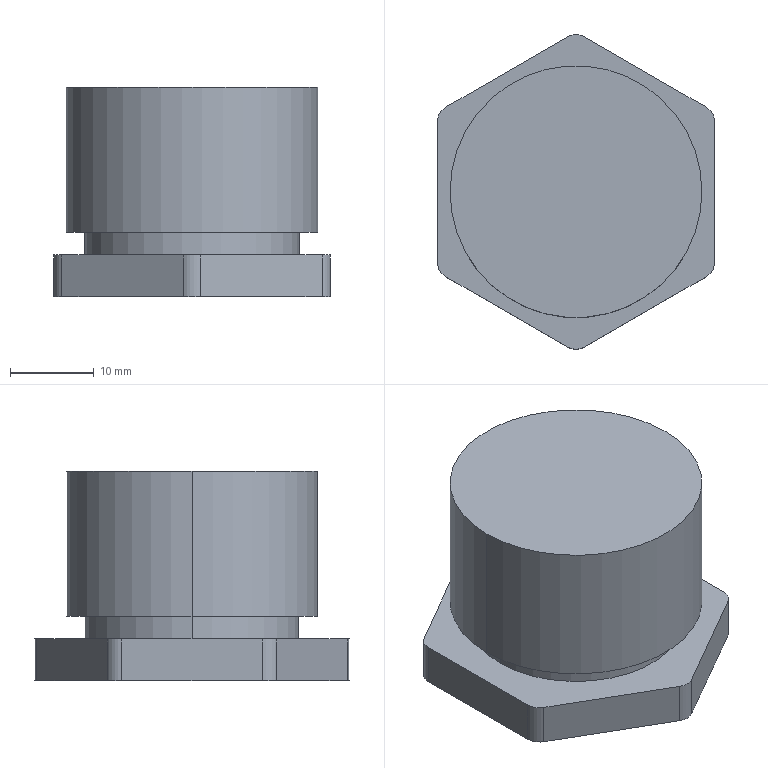Part | STEP file | Feed pipe plug SGN-6-03 | 1 solid | 20 faces | box 33 x 37.486 x 25 mm | volume 18317 mm3 | cylinder 10 | plane 10 | commonest cylinder face diameters 4 x6 25.5 x2 30 x2
STEP:
#1=CARTESIAN_POINT('',(0.,0.,0.));
#2=DIRECTION('',(0.,0.,1.));
#3=DIRECTION('',(1.,0.,0.));
#4=AXIS2_PLACEMENT_3D('',#1,#2,#3);
#5=CARTESIAN_POINT('',(15.,0.,20.));
#6=VERTEX_POINT('',#5);
#7=CARTESIAN_POINT('',(-15.,0.,20.));
#8=VERTEX_POINT('',#7);
#9=CARTESIAN_POINT('',(0.,0.,20.));
#10=DIRECTION('',(0.,0.,1.));
#11=DIRECTION('',(1.,0.,0.));
#12=AXIS2_PLACEMENT_3D('',#9,#10,#11);
#13=CIRCLE('',#12,15.);
#14=CARTESIAN_POINT('',(0.,0.,20.));
#15=DIRECTION('',(0.,0.,-1.));
#16=DIRECTION('',(-1.,0.,0.));
#17=AXIS2_PLACEMENT_3D('',#14,#15,#16);
#18=CYLINDRICAL_SURFACE('',#17,15.);
#19=CARTESIAN_POINT('',(3.142,0.));
#20=DIRECTION('',(-1.,0.));
#21=VECTOR('',#20,1.);
#22=LINE('',#19,#21);
#23=(GEOMETRIC_REPRESENTATION_CONTEXT(2)PARAMETRIC_REPRESENTATION_CONTEXT()REPRESENTATION_CONTEXT('',''));
#24=DEFINITIONAL_REPRESENTATION('',(#22),#23);
#25=PCURVE('',#18,#24);
#26=CARTESIAN_POINT('',(0.,0.,20.));
#27=DIRECTION('',(0.,0.,1.));
#28=DIRECTION('',(1.,0.,0.));
#29=AXIS2_PLACEMENT_3D('',#26,#27,#28);
#30=PLANE('',#29);
#31=CARTESIAN_POINT('',(0.,0.));
#32=DIRECTION('',(1.,0.));
#33=AXIS2_PLACEMENT_2D('',#31,#32);
#34=CIRCLE('',#33,15.);
#35=(GEOMETRIC_REPRESENTATION_CONTEXT(2)PARAMETRIC_REPRESENTATION_CONTEXT()REPRESENTATION_CONTEXT('',''));
#36=DEFINITIONAL_REPRESENTATION('',(#34),#35);
#37=PCURVE('',#30,#36);
#38=SURFACE_CURVE('',#13,(#25,#37),.PCURVE_S1.);
#39=EDGE_CURVE('',#6,#8,#38,.T.);
#40=ORIENTED_EDGE('',*,*,#39,.F.);
#41=CARTESIAN_POINT('',(15.,0.,2.7));
#42=VERTEX_POINT('',#41);
#43=CARTESIAN_POINT('',(15.,0.,20.));
#44=DIRECTION('',(0.,0.,-1.));
#45=VECTOR('',#44,1.);
#46=LINE('',#43,#45);
#47=CARTESIAN_POINT('',(3.142,0.));
#48=DIRECTION('',(0.,1.));
#49=VECTOR('',#48,1.);
#50=LINE('',#47,#49);
#51=(GEOMETRIC_REPRESENTATION_CONTEXT(2)PARAMETRIC_REPRESENTATION_CONTEXT()REPRESENTATION_CONTEXT('',''));
#52=DEFINITIONAL_REPRESENTATION('',(#50),#51);
#53=PCURVE('',#18,#52);
#54=CARTESIAN_POINT('',(0.,0.,20.));
#55=DIRECTION('',(0.,0.,-1.));
#56=DIRECTION('',(-1.,0.,0.));
#57=AXIS2_PLACEMENT_3D('',#54,#55,#56);
#58=CYLINDRICAL_SURFACE('',#57,15.);
#59=CARTESIAN_POINT('',(3.142,0.));
#60=DIRECTION('',(0.,1.));
#61=VECTOR('',#60,1.);
#62=LINE('',#59,#61);
#63=(GEOMETRIC_REPRESENTATION_CONTEXT(2)PARAMETRIC_REPRESENTATION_CONTEXT()REPRESENTATION_CONTEXT('',''));
#64=DEFINITIONAL_REPRESENTATION('',(#62),#63);
#65=PCURVE('',#58,#64);
#66=SURFACE_CURVE('',#46,(#53,#65),.PCURVE_S1.);
#67=EDGE_CURVE('',#6,#42,#66,.T.);
#68=ORIENTED_EDGE('',*,*,#67,.T.);
#69=CARTESIAN_POINT('',(-15.,0.,2.7));
#70=VERTEX_POINT('',#69);
#71=CARTESIAN_POINT('',(0.,0.,2.7));
#72=DIRECTION('',(0.,0.,1.));
#73=DIRECTION('',(1.,0.,0.));
#74=AXIS2_PLACEMENT_3D('',#71,#72,#73);
#75=CIRCLE('',#74,15.);
#76=CARTESIAN_POINT('',(3.142,17.3));
#77=DIRECTION('',(-1.,0.));
#78=VECTOR('',#77,1.);
#79=LINE('',#76,#78);
#80=(GEOMETRIC_REPRESENTATION_CONTEXT(2)PARAMETRIC_REPRESENTATION_CONTEXT()REPRESENTATION_CONTEXT('',''));
#81=DEFINITIONAL_REPRESENTATION('',(#79),#80);
#82=PCURVE('',#18,#81);
#83=CARTESIAN_POINT('',(0.,0.,2.7));
#84=DIRECTION('',(0.,0.,1.));
#85=DIRECTION('',(1.,0.,0.));
#86=AXIS2_PLACEMENT_3D('',#83,#84,#85);
#87=PLANE('',#86);
#88=CARTESIAN_POINT('',(0.,0.));
#89=DIRECTION('',(1.,0.));
#90=AXIS2_PLACEMENT_2D('',#88,#89);
#91=CIRCLE('',#90,15.);
#92=(GEOMETRIC_REPRESENTATION_CONTEXT(2)PARAMETRIC_REPRESENTATION_CONTEXT()REPRESENTATION_CONTEXT('',''));
#93=DEFINITIONAL_REPRESENTATION('',(#91),#92);
#94=PCURVE('',#87,#93);
#95=SURFACE_CURVE('',#75,(#82,#94),.PCURVE_S1.);
#96=EDGE_CURVE('',#42,#70,#95,.T.);
#97=ORIENTED_EDGE('',*,*,#96,.T.);
#98=CARTESIAN_POINT('',(-15.,0.,20.));
#99=DIRECTION('',(0.,0.,-1.));
#100=VECTOR('',#99,1.);
#101=LINE('',#98,#100);
#102=CARTESIAN_POINT('',(0.,0.));
#103=DIRECTION('',(0.,1.));
#104=VECTOR('',#103,1.);
#105=LINE('',#102,#104);
#106=(GEOMETRIC_REPRESENTATION_CONTEXT(2)PARAMETRIC_REPRESENTATION_CONTEXT()REPRESENTATION_CONTEXT('',''));
#107=DEFINITIONAL_REPRESENTATION('',(#105),#106);
#108=PCURVE('',#18,#107);
#109=CARTESIAN_POINT('',(6.283,0.));
#110=DIRECTION('',(0.,1.));
#111=VECTOR('',#110,1.);
#112=LINE('',#109,#111);
#113=(GEOMETRIC_REPRESENTATION_CONTEXT(2)PARAMETRIC_REPRESENTATION_CONTEXT()REPRESENTATION_CONTEXT('',''));
#114=DEFINITIONAL_REPRESENTATION('',(#112),#113);
#115=PCURVE('',#58,#114);
#116=SURFACE_CURVE('',#101,(#108,#115),.PCURVE_S1.);
#117=EDGE_CURVE('',#8,#70,#116,.T.);
#118=ORIENTED_EDGE('',*,*,#117,.F.);
#119=EDGE_LOOP('',(#40,#68,#97,#118));
#120=FACE_BOUND('',#119,.T.);
#121=ADVANCED_FACE('',(#120),#18,.T.);
#122=CARTESIAN_POINT('',(12.75,0.,2.7));
#123=VERTEX_POINT('',#122);
#124=CARTESIAN_POINT('',(-12.75,0.,2.7));
#125=VERTEX_POINT('',#124);
#126=CARTESIAN_POINT('',(0.,0.,2.7));
#127=DIRECTION('',(0.,0.,1.));
#128=DIRECTION('',(1.,0.,0.));
#129=AXIS2_PLACEMENT_3D('',#126,#127,#128);
#130=CIRCLE('',#129,12.75);
#131=CARTESIAN_POINT('',(0.,0.,2.7));
#132=DIRECTION('',(0.,0.,-1.));
#133=DIRECTION('',(-1.,0.,0.));
#134=AXIS2_PLACEMENT_3D('',#131,#132,#133);
#135=CYLINDRICAL_SURFACE('',#134,12.75);
#136=CARTESIAN_POINT('',(3.142,0.));
#137=DIRECTION('',(-1.,0.));
#138=VECTOR('',#137,1.);
#139=LINE('',#136,#138);
#140=(GEOMETRIC_REPRESENTATION_CONTEXT(2)PARAMETRIC_REPRESENTATION_CONTEXT()REPRESENTATION_CONTEXT('',''));
#141=DEFINITIONAL_REPRESENTATION('',(#139),#140);
#142=PCURVE('',#135,#141);
#143=CARTESIAN_POINT('',(0.,0.));
#144=DIRECTION('',(1.,0.));
#145=AXIS2_PLACEMENT_2D('',#143,#144);
#146=CIRCLE('',#145,12.75);
#147=(GEOMETRIC_REPRESENTATION_CONTEXT(2)PARAMETRIC_REPRESENTATION_CONTEXT()REPRESENTATION_CONTEXT('',''));
#148=DEFINITIONAL_REPRESENTATION('',(#146),#147);
#149=PCURVE('',#87,#148);
#150=SURFACE_CURVE('',#130,(#142,#149),.PCURVE_S1.);
#151=EDGE_CURVE('',#123,#125,#150,.T.);
#152=ORIENTED_EDGE('',*,*,#151,.F.);
#153=CARTESIAN_POINT('',(12.75,0.,0.));
#154=VERTEX_POINT('',#153);
#155=CARTESIAN_POINT('',(12.75,0.,2.7));
#156=DIRECTION('',(0.,0.,-1.));
#157=VECTOR('',#156,1.);
#158=LINE('',#155,#157);
#159=CARTESIAN_POINT('',(3.142,0.));
#160=DIRECTION('',(0.,1.));
#161=VECTOR('',#160,1.);
#162=LINE('',#159,#161);
#163=(GEOMETRIC_REPRESENTATION_CONTEXT(2)PARAMETRIC_REPRESENTATION_CONTEXT()REPRESENTATION_CONTEXT('',''));
#164=DEFINITIONAL_REPRESENTATION('',(#162),#163);
#165=PCURVE('',#135,#164);
#166=CARTESIAN_POINT('',(0.,0.,2.7));
#167=DIRECTION('',(0.,0.,-1.));
#168=DIRECTION('',(-1.,0.,0.));
#169=AXIS2_PLACEMENT_3D('',#166,#167,#168);
#170=CYLINDRICAL_SURFACE('',#169,12.75);
#171=CARTESIAN_POINT('',(3.142,0.));
#172=DIRECTION('',(0.,1.));
#173=VECTOR('',#172,1.);
#174=LINE('',#171,#173);
#175=(GEOMETRIC_REPRESENTATION_CONTEXT(2)PARAMETRIC_REPRESENTATION_CONTEXT()REPRESENTATION_CONTEXT('',''));
#176=DEFINITIONAL_REPRESENTATION('',(#174),#175);
#177=PCURVE('',#170,#176);
#178=SURFACE_CURVE('',#158,(#165,#177),.PCURVE_S1.);
#179=EDGE_CURVE('',#123,#154,#178,.T.);
#180=ORIENTED_EDGE('',*,*,#179,.T.);
#181=CARTESIAN_POINT('',(-12.75,0.,0.));
#182=VERTEX_POINT('',#181);
#183=CARTESIAN_POINT('',(0.,0.,0.));
#184=DIRECTION('',(0.,0.,1.));
#185=DIRECTION('',(1.,0.,0.));
#186=AXIS2_PLACEMENT_3D('',#183,#184,#185);
#187=CIRCLE('',#186,12.75);
#188=CARTESIAN_POINT('',(3.142,2.7));
#189=DIRECTION('',(-1.,0.));
#190=VECTOR('',#189,1.);
#191=LINE('',#188,#190);
#192=(GEOMETRIC_REPRESENTATION_CONTEXT(2)PARAMETRIC_REPRESENTATION_CONTEXT()REPRESENTATION_CONTEXT('',''));
#193=DEFINITIONAL_REPRESENTATION('',(#191),#192);
#194=PCURVE('',#135,#193);
#195=CARTESIAN_POINT('',(0.,0.,0.));
#196=DIRECTION('',(0.,0.,-1.));
#197=DIRECTION('',(-1.,0.,0.));
#198=AXIS2_PLACEMENT_3D('',#195,#196,#197);
#199=PLANE('',#198);
#200=CARTESIAN_POINT('',(-12.75,0.));
#201=CARTESIAN_POINT('',(-12.75,22.084));
#202=CARTESIAN_POINT('',(6.375,11.042));
#203=CARTESIAN_POINT('',(25.5,0.));
#204=CARTESIAN_POINT('',(6.375,-11.042));
#205=CARTESIAN_POINT('',(-12.75,-22.084));
#206=CARTESIAN_POINT('',(-12.75,0.));
#207=(BOUNDED_CURVE()B_SPLINE_CURVE(2,(#200,#201,#202,#203,#204,#205,#206),.UNSPECIFIED.,.T.,.F.)B_SPLINE_CURVE_WITH_KNOTS((1,2,2,2,2,1),(-2.094,0.,2.094,4.189,6.283,8.378),.UNSPECIFIED.)CURVE()GEOMETRIC_REPRESENTATION_ITEM()RATIONAL_B_SPLINE_CURVE((1.,0.5,1.,0.5,1.,0.5,1.))REPRESENTATION_ITEM(''));
#208=(GEOMETRIC_REPRESENTATION_CONTEXT(2)PARAMETRIC_REPRESENTATION_CONTEXT()REPRESENTATION_CONTEXT('',''));
#209=DEFINITIONAL_REPRESENTATION('',(#207),#208);
#210=PCURVE('',#199,#209);
#211=SURFACE_CURVE('',#187,(#194,#210),.PCURVE_S1.);
#212=EDGE_CURVE('',#154,#182,#211,.T.);
#213=ORIENTED_EDGE('',*,*,#212,.T.);
#214=CARTESIAN_POINT('',(-12.75,0.,2.7));
#215=DIRECTION('',(0.,0.,-1.));
#216=VECTOR('',#215,1.);
#217=LINE('',#214,#216);
#218=CARTESIAN_POINT('',(0.,0.));
#219=DIRECTION('',(0.,1.));
#220=VECTOR('',#219,1.);
#221=LINE('',#218,#220);
#222=(GEOMETRIC_REPRESENTATION_CONTEXT(2)PARAMETRIC_REPRESENTATION_CONTEXT()REPRESENTATION_CONTEXT('',''));
#223=DEFINITIONAL_REPRESENTATION('',(#221),#222);
#224=PCURVE('',#135,#223);
#225=CARTESIAN_POINT('',(6.283,0.));
#226=DIRECTION('',(0.,1.));
#227=VECTOR('',#226,1.);
#228=LINE('',#225,#227);
#229=(GEOMETRIC_REPRESENTATION_CONTEXT(2)PARAMETRIC_REPRESENTATION_CONTEXT()REPRESENTATION_CONTEXT('',''));
#230=DEFINITIONAL_REPRESENTATION('',(#228),#229);
#231=PCURVE('',#170,#230);
#232=SURFACE_CURVE('',#217,(#224,#231),.PCURVE_S1.);
#233=EDGE_CURVE('',#125,#182,#232,.T.);
#234=ORIENTED_EDGE('',*,*,#233,.F.);
#235=EDGE_LOOP('',(#152,#180,#213,#234));
#236=FACE_BOUND('',#235,.T.);
#237=ADVANCED_FACE('',(#236),#135,.T.);
#238=CARTESIAN_POINT('',(-15.5,10.104,-5.));
#239=VERTEX_POINT('',#238);
#240=CARTESIAN_POINT('',(-1.,18.475,-5.));
#241=VERTEX_POINT('',#240);
#242=CARTESIAN_POINT('',(-16.5,9.526,-5.));
#243=DIRECTION('',(0.866,0.5,0.));
#244=VECTOR('',#243,1.);
#245=LINE('',#242,#244);
#246=CARTESIAN_POINT('',(-16.5,9.526,-5.));
#247=DIRECTION('',(0.5,-0.866,0.));
#248=DIRECTION('',(0.866,0.5,0.));
#249=AXIS2_PLACEMENT_3D('',#246,#247,#248);
#250=PLANE('',#249);
#251=CARTESIAN_POINT('',(0.,0.));
#252=DIRECTION('',(1.,0.));
#253=VECTOR('',#252,1.);
#254=LINE('',#251,#253);
#255=(GEOMETRIC_REPRESENTATION_CONTEXT(2)PARAMETRIC_REPRESENTATION_CONTEXT()REPRESENTATION_CONTEXT('',''));
#256=DEFINITIONAL_REPRESENTATION('',(#254),#255);
#257=PCURVE('',#250,#256);
#258=CARTESIAN_POINT('',(0.,0.,-5.));
#259=DIRECTION('',(0.,0.,-1.));
#260=DIRECTION('',(-1.,0.,0.));
#261=AXIS2_PLACEMENT_3D('',#258,#259,#260);
#262=PLANE('',#261);
#263=CARTESIAN_POINT('',(16.5,9.526));
#264=DIRECTION('',(-0.866,0.5));
#265=VECTOR('',#264,1.);
#266=LINE('',#263,#265);
#267=(GEOMETRIC_REPRESENTATION_CONTEXT(2)PARAMETRIC_REPRESENTATION_CONTEXT()REPRESENTATION_CONTEXT('',''));
#268=DEFINITIONAL_REPRESENTATION('',(#266),#267);
#269=PCURVE('',#262,#268);
#270=SURFACE_CURVE('',#245,(#257,#269),.PCURVE_S1.);
#271=EDGE_CURVE('',#239,#241,#270,.T.);
#272=ORIENTED_EDGE('',*,*,#271,.F.);
#273=CARTESIAN_POINT('',(-15.5,10.104,0.));
#274=VERTEX_POINT('',#273);
#275=CARTESIAN_POINT('',(-15.5,10.104,-5.));
#276=DIRECTION('',(0.,0.,1.));
#277=VECTOR('',#276,1.);
#278=LINE('',#275,#277);
#279=CARTESIAN_POINT('',(1.155,0.));
#280=DIRECTION('',(0.,1.));
#281=VECTOR('',#280,1.);
#282=LINE('',#279,#281);
#283=(GEOMETRIC_REPRESENTATION_CONTEXT(2)PARAMETRIC_REPRESENTATION_CONTEXT()REPRESENTATION_CONTEXT('',''));
#284=DEFINITIONAL_REPRESENTATION('',(#282),#283);
#285=PCURVE('',#250,#284);
#286=CARTESIAN_POINT('',(-14.5,8.372,-5.));
#287=DIRECTION('',(0.,0.,1.));
#288=DIRECTION('',(1.,0.,0.));
#289=AXIS2_PLACEMENT_3D('',#286,#287,#288);
#290=CYLINDRICAL_SURFACE('',#289,2.);
#291=CARTESIAN_POINT('',(2.094,0.));
#292=DIRECTION('',(0.,1.));
#293=VECTOR('',#292,1.);
#294=LINE('',#291,#293);
#295=(GEOMETRIC_REPRESENTATION_CONTEXT(2)PARAMETRIC_REPRESENTATION_CONTEXT()REPRESENTATION_CONTEXT('',''));
#296=DEFINITIONAL_REPRESENTATION('',(#294),#295);
#297=PCURVE('',#290,#296);
#298=SURFACE_CURVE('',#278,(#285,#297),.PCURVE_S1.);
#299=EDGE_CURVE('',#239,#274,#298,.T.);
#300=ORIENTED_EDGE('',*,*,#299,.T.);
#301=CARTESIAN_POINT('',(-1.,18.475,0.));
#302=VERTEX_POINT('',#301);
#303=CARTESIAN_POINT('',(-16.5,9.526,0.));
#304=DIRECTION('',(0.866,0.5,0.));
#305=VECTOR('',#304,1.);
#306=LINE('',#303,#305);
#307=CARTESIAN_POINT('',(0.,5.));
#308=DIRECTION('',(1.,0.));
#309=VECTOR('',#308,1.);
#310=LINE('',#307,#309);
#311=(GEOMETRIC_REPRESENTATION_CONTEXT(2)PARAMETRIC_REPRESENTATION_CONTEXT()REPRESENTATION_CONTEXT('',''));
#312=DEFINITIONAL_REPRESENTATION('',(#310),#311);
#313=PCURVE('',#250,#312);
#314=CARTESIAN_POINT('',(16.5,9.526));
#315=DIRECTION('',(-0.866,0.5));
#316=VECTOR('',#315,1.);
#317=LINE('',#314,#316);
#318=(GEOMETRIC_REPRESENTATION_CONTEXT(2)PARAMETRIC_REPRESENTATION_CONTEXT()REPRESENTATION_CONTEXT('',''));
#319=DEFINITIONAL_REPRESENTATION('',(#317),#318);
#320=PCURVE('',#199,#319);
#321=SURFACE_CURVE('',#306,(#313,#320),.PCURVE_S1.);
#322=EDGE_CURVE('',#274,#302,#321,.T.);
#323=ORIENTED_EDGE('',*,*,#322,.T.);
#324=CARTESIAN_POINT('',(-1.,18.475,-5.));
#325=DIRECTION('',(0.,0.,-1.));
#326=VECTOR('',#325,1.);
#327=LINE('',#324,#326);
#328=CARTESIAN_POINT('',(17.898,0.));
#329=DIRECTION('',(0.,-1.));
#330=VECTOR('',#329,1.);
#331=LINE('',#328,#330);
#332=(GEOMETRIC_REPRESENTATION_CONTEXT(2)PARAMETRIC_REPRESENTATION_CONTEXT()REPRESENTATION_CONTEXT('',''));
#333=DEFINITIONAL_REPRESENTATION('',(#331),#332);
#334=PCURVE('',#250,#333);
#335=CARTESIAN_POINT('',(0.,16.743,-5.));
#336=DIRECTION('',(0.,0.,1.));
#337=DIRECTION('',(1.,0.,0.));
#338=AXIS2_PLACEMENT_3D('',#335,#336,#337);
#339=CYLINDRICAL_SURFACE('',#338,2.);
#340=CARTESIAN_POINT('',(2.094,0.));
#341=DIRECTION('',(0.,-1.));
#342=VECTOR('',#341,1.);
#343=LINE('',#340,#342);
#344=(GEOMETRIC_REPRESENTATION_CONTEXT(2)PARAMETRIC_REPRESENTATION_CONTEXT()REPRESENTATION_CONTEXT('',''));
#345=DEFINITIONAL_REPRESENTATION('',(#343),#344);
#346=PCURVE('',#339,#345);
#347=SURFACE_CURVE('',#327,(#334,#346),.PCURVE_S1.);
#348=EDGE_CURVE('',#302,#241,#347,.T.);
#349=ORIENTED_EDGE('',*,*,#348,.T.);
#350=EDGE_LOOP('',(#272,#300,#323,#349));
#351=FACE_BOUND('',#350,.T.);
#352=ADVANCED_FACE('',(#351),#250,.F.);
#353=CARTESIAN_POINT('',(1.,18.475,0.));
#354=VERTEX_POINT('',#353);
#355=CARTESIAN_POINT('',(15.5,10.104,0.));
#356=VERTEX_POINT('',#355);
#357=CARTESIAN_POINT('',(0.,19.053,0.));
#358=DIRECTION('',(0.866,-0.5,0.));
#359=VECTOR('',#358,1.);
#360=LINE('',#357,#359);
#361=CARTESIAN_POINT('',(0.,19.053,-5.));
#362=DIRECTION('',(-0.5,-0.866,0.));
#363=DIRECTION('',(0.866,-0.5,0.));
#364=AXIS2_PLACEMENT_3D('',#361,#362,#363);
#365=PLANE('',#364);
#366=CARTESIAN_POINT('',(0.,5.));
#367=DIRECTION('',(1.,0.));
#368=VECTOR('',#367,1.);
#369=LINE('',#366,#368);
#370=(GEOMETRIC_REPRESENTATION_CONTEXT(2)PARAMETRIC_REPRESENTATION_CONTEXT()REPRESENTATION_CONTEXT('',''));
#371=DEFINITIONAL_REPRESENTATION('',(#369),#370);
#372=PCURVE('',#365,#371);
#373=CARTESIAN_POINT('',(0.,19.053));
#374=DIRECTION('',(-0.866,-0.5));
#375=VECTOR('',#374,1.);
#376=LINE('',#373,#375);
#377=(GEOMETRIC_REPRESENTATION_CONTEXT(2)PARAMETRIC_REPRESENTATION_CONTEXT()REPRESENTATION_CONTEXT('',''));
#378=DEFINITIONAL_REPRESENTATION('',(#376),#377);
#379=PCURVE('',#199,#378);
#380=SURFACE_CURVE('',#360,(#372,#379),.PCURVE_S1.);
#381=EDGE_CURVE('',#354,#356,#380,.T.);
#382=ORIENTED_EDGE('',*,*,#381,.T.);
#383=CARTESIAN_POINT('',(15.5,10.104,-5.));
#384=VERTEX_POINT('',#383);
#385=CARTESIAN_POINT('',(15.5,10.104,-5.));
#386=DIRECTION('',(0.,0.,-1.));
#387=VECTOR('',#386,1.);
#388=LINE('',#385,#387);
#389=CARTESIAN_POINT('',(17.898,0.));
#390=DIRECTION('',(0.,-1.));
#391=VECTOR('',#390,1.);
#392=LINE('',#389,#391);
#393=(GEOMETRIC_REPRESENTATION_CONTEXT(2)PARAMETRIC_REPRESENTATION_CONTEXT()REPRESENTATION_CONTEXT('',''));
#394=DEFINITIONAL_REPRESENTATION('',(#392),#393);
#395=PCURVE('',#365,#394);
#396=CARTESIAN_POINT('',(14.5,8.372,-5.));
#397=DIRECTION('',(0.,0.,1.));
#398=DIRECTION('',(1.,0.,0.));
#399=AXIS2_PLACEMENT_3D('',#396,#397,#398);
#400=CYLINDRICAL_SURFACE('',#399,2.);
#401=CARTESIAN_POINT('',(1.047,0.));
#402=DIRECTION('',(0.,-1.));
#403=VECTOR('',#402,1.);
#404=LINE('',#401,#403);
#405=(GEOMETRIC_REPRESENTATION_CONTEXT(2)PARAMETRIC_REPRESENTATION_CONTEXT()REPRESENTATION_CONTEXT('',''));
#406=DEFINITIONAL_REPRESENTATION('',(#404),#405);
#407=PCURVE('',#400,#406);
#408=SURFACE_CURVE('',#388,(#395,#407),.PCURVE_S1.);
#409=EDGE_CURVE('',#356,#384,#408,.T.);
#410=ORIENTED_EDGE('',*,*,#409,.T.);
#411=CARTESIAN_POINT('',(1.,18.475,-5.));
#412=VERTEX_POINT('',#411);
#413=CARTESIAN_POINT('',(0.,19.053,-5.));
#414=DIRECTION('',(0.866,-0.5,0.));
#415=VECTOR('',#414,1.);
#416=LINE('',#413,#415);
#417=CARTESIAN_POINT('',(0.,0.));
#418=DIRECTION('',(1.,0.));
#419=VECTOR('',#418,1.);
#420=LINE('',#417,#419);
#421=(GEOMETRIC_REPRESENTATION_CONTEXT(2)PARAMETRIC_REPRESENTATION_CONTEXT()REPRESENTATION_CONTEXT('',''));
#422=DEFINITIONAL_REPRESENTATION('',(#420),#421);
#423=PCURVE('',#365,#422);
#424=CARTESIAN_POINT('',(0.,19.053));
#425=DIRECTION('',(-0.866,-0.5));
#426=VECTOR('',#425,1.);
#427=LINE('',#424,#426);
#428=(GEOMETRIC_REPRESENTATION_CONTEXT(2)PARAMETRIC_REPRESENTATION_CONTEXT()REPRESENTATION_CONTEXT('',''));
#429=DEFINITIONAL_REPRESENTATION('',(#427),#428);
#430=PCURVE('',#262,#429);
#431=SURFACE_CURVE('',#416,(#423,#430),.PCURVE_S1.);
#432=EDGE_CURVE('',#412,#384,#431,.T.);
#433=ORIENTED_EDGE('',*,*,#432,.F.);
#434=CARTESIAN_POINT('',(1.,18.475,-5.));
#435=DIRECTION('',(0.,0.,1.));
#436=VECTOR('',#435,1.);
#437=LINE('',#434,#436);
#438=CARTESIAN_POINT('',(1.155,0.));
#439=DIRECTION('',(0.,1.));
#440=VECTOR('',#439,1.);
#441=LINE('',#438,#440);
#442=(GEOMETRIC_REPRESENTATION_CONTEXT(2)PARAMETRIC_REPRESENTATION_CONTEXT()REPRESENTATION_CONTEXT('',''));
#443=DEFINITIONAL_REPRESENTATION('',(#441),#442);
#444=PCURVE('',#365,#443);
#445=CARTESIAN_POINT('',(1.047,0.));
#446=DIRECTION('',(0.,1.));
#447=VECTOR('',#446,1.);
#448=LINE('',#445,#447);
#449=(GEOMETRIC_REPRESENTATION_CONTEXT(2)PARAMETRIC_REPRESENTATION_CONTEXT()REPRESENTATION_CONTEXT('',''));
#450=DEFINITIONAL_REPRESENTATION('',(#448),#449);
#451=PCURVE('',#339,#450);
#452=SURFACE_CURVE('',#437,(#444,#451),.PCURVE_S1.);
#453=EDGE_CURVE('',#412,#354,#452,.T.);
#454=ORIENTED_EDGE('',*,*,#453,.T.);
#455=EDGE_LOOP('',(#382,#410,#433,#454));
#456=FACE_BOUND('',#455,.T.);
#457=ADVANCED_FACE('',(#456),#365,.F.);
#458=CARTESIAN_POINT('',(16.5,8.372,-5.));
#459=VERTEX_POINT('',#458);
#460=CARTESIAN_POINT('',(16.5,-8.372,-5.));
#461=VERTEX_POINT('',#460);
#462=CARTESIAN_POINT('',(16.5,9.526,-5.));
#463=DIRECTION('',(0.,-1.,0.));
#464=VECTOR('',#463,1.);
#465=LINE('',#462,#464);
#466=CARTESIAN_POINT('',(16.5,9.526,-5.));
#467=DIRECTION('',(-1.,0.,0.));
#468=DIRECTION('',(0.,-1.,0.));
#469=AXIS2_PLACEMENT_3D('',#466,#467,#468);
#470=PLANE('',#469);
#471=CARTESIAN_POINT('',(0.,0.));
#472=DIRECTION('',(1.,0.));
#473=VECTOR('',#472,1.);
#474=LINE('',#471,#473);
#475=(GEOMETRIC_REPRESENTATION_CONTEXT(2)PARAMETRIC_REPRESENTATION_CONTEXT()REPRESENTATION_CONTEXT('',''));
#476=DEFINITIONAL_REPRESENTATION('',(#474),#475);
#477=PCURVE('',#470,#476);
#478=CARTESIAN_POINT('',(-16.5,9.526));
#479=DIRECTION('',(0.,-1.));
#480=VECTOR('',#479,1.);
#481=LINE('',#478,#480);
#482=(GEOMETRIC_REPRESENTATION_CONTEXT(2)PARAMETRIC_REPRESENTATION_CONTEXT()REPRESENTATION_CONTEXT('',''));
#483=DEFINITIONAL_REPRESENTATION('',(#481),#482);
#484=PCURVE('',#262,#483);
#485=SURFACE_CURVE('',#465,(#477,#484),.PCURVE_S1.);
#486=EDGE_CURVE('',#459,#461,#485,.T.);
#487=ORIENTED_EDGE('',*,*,#486,.F.);
#488=CARTESIAN_POINT('',(16.5,8.372,0.));
#489=VERTEX_POINT('',#488);
#490=CARTESIAN_POINT('',(16.5,8.372,-5.));
#491=DIRECTION('',(0.,0.,1.));
#492=VECTOR('',#491,1.);
#493=LINE('',#490,#492);
#494=CARTESIAN_POINT('',(1.155,0.));
#495=DIRECTION('',(0.,1.));
#496=VECTOR('',#495,1.);
#497=LINE('',#494,#496);
#498=(GEOMETRIC_REPRESENTATION_CONTEXT(2)PARAMETRIC_REPRESENTATION_CONTEXT()REPRESENTATION_CONTEXT('',''));
#499=DEFINITIONAL_REPRESENTATION('',(#497),#498);
#500=PCURVE('',#470,#499);
#501=CARTESIAN_POINT('',(0.,0.));
#502=DIRECTION('',(0.,1.));
#503=VECTOR('',#502,1.);
#504=LINE('',#501,#503);
#505=(GEOMETRIC_REPRESENTATION_CONTEXT(2)PARAMETRIC_REPRESENTATION_CONTEXT()REPRESENTATION_CONTEXT('',''));
#506=DEFINITIONAL_REPRESENTATION('',(#504),#505);
#507=PCURVE('',#400,#506);
#508=SURFACE_CURVE('',#493,(#500,#507),.PCURVE_S1.);
#509=EDGE_CURVE('',#459,#489,#508,.T.);
#510=ORIENTED_EDGE('',*,*,#509,.T.);
#511=CARTESIAN_POINT('',(16.5,-8.372,0.));
#512=VERTEX_POINT('',#511);
#513=CARTESIAN_POINT('',(16.5,9.526,0.));
#514=DIRECTION('',(0.,-1.,0.));
#515=VECTOR('',#514,1.);
#516=LINE('',#513,#515);
#517=CARTESIAN_POINT('',(0.,5.));
#518=DIRECTION('',(1.,0.));
#519=VECTOR('',#518,1.);
#520=LINE('',#517,#519);
#521=(GEOMETRIC_REPRESENTATION_CONTEXT(2)PARAMETRIC_REPRESENTATION_CONTEXT()REPRESENTATION_CONTEXT('',''));
#522=DEFINITIONAL_REPRESENTATION('',(#520),#521);
#523=PCURVE('',#470,#522);
#524=CARTESIAN_POINT('',(-16.5,9.526));
#525=DIRECTION('',(0.,-1.));
#526=VECTOR('',#525,1.);
#527=LINE('',#524,#526);
#528=(GEOMETRIC_REPRESENTATION_CONTEXT(2)PARAMETRIC_REPRESENTATION_CONTEXT()REPRESENTATION_CONTEXT('',''));
#529=DEFINITIONAL_REPRESENTATION('',(#527),#528);
#530=PCURVE('',#199,#529);
#531=SURFACE_CURVE('',#516,(#523,#530),.PCURVE_S1.);
#532=EDGE_CURVE('',#489,#512,#531,.T.);
#533=ORIENTED_EDGE('',*,*,#532,.T.);
#534=CARTESIAN_POINT('',(16.5,-8.372,-5.));
#535=DIRECTION('',(0.,0.,-1.));
#536=VECTOR('',#535,1.);
#537=LINE('',#534,#536);
#538=CARTESIAN_POINT('',(17.898,0.));
#539=DIRECTION('',(0.,-1.));
#540=VECTOR('',#539,1.);
#541=LINE('',#538,#540);
#542=(GEOMETRIC_REPRESENTATION_CONTEXT(2)PARAMETRIC_REPRESENTATION_CONTEXT()REPRESENTATION_CONTEXT('',''));
#543=DEFINITIONAL_REPRESENTATION('',(#541),#542);
#544=PCURVE('',#470,#543);
#545=CARTESIAN_POINT('',(14.5,-8.372,-5.));
#546=DIRECTION('',(0.,0.,1.));
#547=DIRECTION('',(1.,0.,0.));
#548=AXIS2_PLACEMENT_3D('',#545,#546,#547);
#549=CYLINDRICAL_SURFACE('',#548,2.);
#550=CARTESIAN_POINT('',(6.283,0.));
#551=DIRECTION('',(0.,-1.));
#552=VECTOR('',#551,1.);
#553=LINE('',#550,#552);
#554=(GEOMETRIC_REPRESENTATION_CONTEXT(2)PARAMETRIC_REPRESENTATION_CONTEXT()REPRESENTATION_CONTEXT('',''));
#555=DEFINITIONAL_REPRESENTATION('',(#553),#554);
#556=PCURVE('',#549,#555);
#557=SURFACE_CURVE('',#537,(#544,#556),.PCURVE_S1.);
#558=EDGE_CURVE('',#512,#461,#557,.T.);
#559=ORIENTED_EDGE('',*,*,#558,.T.);
#560=EDGE_LOOP('',(#487,#510,#533,#559));
#561=FACE_BOUND('',#560,.T.);
#562=ADVANCED_FACE('',(#561),#470,.F.);
#563=CARTESIAN_POINT('',(15.5,-10.104,-5.));
#564=VERTEX_POINT('',#563);
#565=CARTESIAN_POINT('',(1.,-18.475,-5.));
#566=VERTEX_POINT('',#565);
#567=CARTESIAN_POINT('',(16.5,-9.526,-5.));
#568=DIRECTION('',(-0.866,-0.5,0.));
#569=VECTOR('',#568,1.);
#570=LINE('',#567,#569);
#571=CARTESIAN_POINT('',(16.5,-9.526,-5.));
#572=DIRECTION('',(-0.5,0.866,0.));
#573=DIRECTION('',(-0.866,-0.5,0.));
#574=AXIS2_PLACEMENT_3D('',#571,#572,#573);
#575=PLANE('',#574);
#576=CARTESIAN_POINT('',(0.,0.));
#577=DIRECTION('',(1.,0.));
#578=VECTOR('',#577,1.);
#579=LINE('',#576,#578);
#580=(GEOMETRIC_REPRESENTATION_CONTEXT(2)PARAMETRIC_REPRESENTATION_CONTEXT()REPRESENTATION_CONTEXT('',''));
#581=DEFINITIONAL_REPRESENTATION('',(#579),#580);
#582=PCURVE('',#575,#581);
#583=CARTESIAN_POINT('',(-16.5,-9.526));
#584=DIRECTION('',(0.866,-0.5));
#585=VECTOR('',#584,1.);
#586=LINE('',#583,#585);
#587=(GEOMETRIC_REPRESENTATION_CONTEXT(2)PARAMETRIC_REPRESENTATION_CONTEXT()REPRESENTATION_CONTEXT('',''));
#588=DEFINITIONAL_REPRESENTATION('',(#586),#587);
#589=PCURVE('',#262,#588);
#590=SURFACE_CURVE('',#570,(#582,#589),.PCURVE_S1.);
#591=EDGE_CURVE('',#564,#566,#590,.T.);
#592=ORIENTED_EDGE('',*,*,#591,.F.);
#593=CARTESIAN_POINT('',(15.5,-10.104,0.));
#594=VERTEX_POINT('',#593);
#595=CARTESIAN_POINT('',(15.5,-10.104,-5.));
#596=DIRECTION('',(0.,0.,1.));
#597=VECTOR('',#596,1.);
#598=LINE('',#595,#597);
#599=CARTESIAN_POINT('',(1.155,0.));
#600=DIRECTION('',(0.,1.));
#601=VECTOR('',#600,1.);
#602=LINE('',#599,#601);
#603=(GEOMETRIC_REPRESENTATION_CONTEXT(2)PARAMETRIC_REPRESENTATION_CONTEXT()REPRESENTATION_CONTEXT('',''));
#604=DEFINITIONAL_REPRESENTATION('',(#602),#603);
#605=PCURVE('',#575,#604);
#606=CARTESIAN_POINT('',(5.236,0.));
#607=DIRECTION('',(0.,1.));
#608=VECTOR('',#607,1.);
#609=LINE('',#606,#608);
#610=(GEOMETRIC_REPRESENTATION_CONTEXT(2)PARAMETRIC_REPRESENTATION_CONTEXT()REPRESENTATION_CONTEXT('',''));
#611=DEFINITIONAL_REPRESENTATION('',(#609),#610);
#612=PCURVE('',#549,#611);
#613=SURFACE_CURVE('',#598,(#605,#612),.PCURVE_S1.);
#614=EDGE_CURVE('',#564,#594,#613,.T.);
#615=ORIENTED_EDGE('',*,*,#614,.T.);
#616=CARTESIAN_POINT('',(1.,-18.475,0.));
#617=VERTEX_POINT('',#616);
#618=CARTESIAN_POINT('',(16.5,-9.526,0.));
#619=DIRECTION('',(-0.866,-0.5,0.));
#620=VECTOR('',#619,1.);
#621=LINE('',#618,#620);
#622=CARTESIAN_POINT('',(0.,5.));
#623=DIRECTION('',(1.,0.));
#624=VECTOR('',#623,1.);
#625=LINE('',#622,#624);
#626=(GEOMETRIC_REPRESENTATION_CONTEXT(2)PARAMETRIC_REPRESENTATION_CONTEXT()REPRESENTATION_CONTEXT('',''));
#627=DEFINITIONAL_REPRESENTATION('',(#625),#626);
#628=PCURVE('',#575,#627);
#629=CARTESIAN_POINT('',(-16.5,-9.526));
#630=DIRECTION('',(0.866,-0.5));
#631=VECTOR('',#630,1.);
#632=LINE('',#629,#631);
#633=(GEOMETRIC_REPRESENTATION_CONTEXT(2)PARAMETRIC_REPRESENTATION_CONTEXT()REPRESENTATION_CONTEXT('',''));
#634=DEFINITIONAL_REPRESENTATION('',(#632),#633);
#635=PCURVE('',#199,#634);
#636=SURFACE_CURVE('',#621,(#628,#635),.PCURVE_S1.);
#637=EDGE_CURVE('',#594,#617,#636,.T.);
#638=ORIENTED_EDGE('',*,*,#637,.T.);
#639=CARTESIAN_POINT('',(1.,-18.475,-5.));
#640=DIRECTION('',(0.,0.,-1.));
#641=VECTOR('',#640,1.);
#642=LINE('',#639,#641);
#643=CARTESIAN_POINT('',(17.898,0.));
#644=DIRECTION('',(0.,-1.));
#645=VECTOR('',#644,1.);
#646=LINE('',#643,#645);
#647=(GEOMETRIC_REPRESENTATION_CONTEXT(2)PARAMETRIC_REPRESENTATION_CONTEXT()REPRESENTATION_CONTEXT('',''));
#648=DEFINITIONAL_REPRESENTATION('',(#646),#647);
#649=PCURVE('',#575,#648);
#650=CARTESIAN_POINT('',(0.,-16.743,-5.));
#651=DIRECTION('',(0.,0.,1.));
#652=DIRECTION('',(1.,0.,0.));
#653=AXIS2_PLACEMENT_3D('',#650,#651,#652);
#654=CYLINDRICAL_SURFACE('',#653,2.);
#655=CARTESIAN_POINT('',(5.236,0.));
#656=DIRECTION('',(0.,-1.));
#657=VECTOR('',#656,1.);
#658=LINE('',#655,#657);
#659=(GEOMETRIC_REPRESENTATION_CONTEXT(2)PARAMETRIC_REPRESENTATION_CONTEXT()REPRESENTATION_CONTEXT('',''));
#660=DEFINITIONAL_REPRESENTATION('',(#658),#659);
#661=PCURVE('',#654,#660);
#662=SURFACE_CURVE('',#642,(#649,#661),.PCURVE_S1.);
#663=EDGE_CURVE('',#617,#566,#662,.T.);
#664=ORIENTED_EDGE('',*,*,#663,.T.);
#665=EDGE_LOOP('',(#592,#615,#638,#664));
#666=FACE_BOUND('',#665,.T.);
#667=ADVANCED_FACE('',(#666),#575,.F.);
#668=CARTESIAN_POINT('',(-1.,-18.475,-5.));
#669=VERTEX_POINT('',#668);
#670=CARTESIAN_POINT('',(-15.5,-10.104,-5.));
#671=VERTEX_POINT('',#670);
#672=CARTESIAN_POINT('',(0.,-19.053,-5.));
#673=DIRECTION('',(-0.866,0.5,0.));
#674=VECTOR('',#673,1.);
#675=LINE('',#672,#674);
#676=CARTESIAN_POINT('',(0.,-19.053,-5.));
#677=DIRECTION('',(0.5,0.866,0.));
#678=DIRECTION('',(-0.866,0.5,0.));
#679=AXIS2_PLACEMENT_3D('',#676,#677,#678);
#680=PLANE('',#679);
#681=CARTESIAN_POINT('',(0.,0.));
#682=DIRECTION('',(1.,0.));
#683=VECTOR('',#682,1.);
#684=LINE('',#681,#683);
#685=(GEOMETRIC_REPRESENTATION_CONTEXT(2)PARAMETRIC_REPRESENTATION_CONTEXT()REPRESENTATION_CONTEXT('',''));
#686=DEFINITIONAL_REPRESENTATION('',(#684),#685);
#687=PCURVE('',#680,#686);
#688=CARTESIAN_POINT('',(0.,-19.053));
#689=DIRECTION('',(0.866,0.5));
#690=VECTOR('',#689,1.);
#691=LINE('',#688,#690);
#692=(GEOMETRIC_REPRESENTATION_CONTEXT(2)PARAMETRIC_REPRESENTATION_CONTEXT()REPRESENTATION_CONTEXT('',''));
#693=DEFINITIONAL_REPRESENTATION('',(#691),#692);
#694=PCURVE('',#262,#693);
#695=SURFACE_CURVE('',#675,(#687,#694),.PCURVE_S1.);
#696=EDGE_CURVE('',#669,#671,#695,.T.);
#697=ORIENTED_EDGE('',*,*,#696,.F.);
#698=CARTESIAN_POINT('',(-1.,-18.475,0.));
#699=VERTEX_POINT('',#698);
#700=CARTESIAN_POINT('',(-1.,-18.475,-5.));
#701=DIRECTION('',(0.,0.,1.));
#702=VECTOR('',#701,1.);
#703=LINE('',#700,#702);
#704=CARTESIAN_POINT('',(1.155,0.));
#705=DIRECTION('',(0.,1.));
#706=VECTOR('',#705,1.);
#707=LINE('',#704,#706);
#708=(GEOMETRIC_REPRESENTATION_CONTEXT(2)PARAMETRIC_REPRESENTATION_CONTEXT()REPRESENTATION_CONTEXT('',''));
#709=DEFINITIONAL_REPRESENTATION('',(#707),#708);
#710=PCURVE('',#680,#709);
#711=CARTESIAN_POINT('',(4.189,0.));
#712=DIRECTION('',(0.,1.));
#713=VECTOR('',#712,1.);
#714=LINE('',#711,#713);
#715=(GEOMETRIC_REPRESENTATION_CONTEXT(2)PARAMETRIC_REPRESENTATION_CONTEXT()REPRESENTATION_CONTEXT('',''));
#716=DEFINITIONAL_REPRESENTATION('',(#714),#715);
#717=PCURVE('',#654,#716);
#718=SURFACE_CURVE('',#703,(#710,#717),.PCURVE_S1.);
#719=EDGE_CURVE('',#669,#699,#718,.T.);
#720=ORIENTED_EDGE('',*,*,#719,.T.);
#721=CARTESIAN_POINT('',(-15.5,-10.104,0.));
#722=VERTEX_POINT('',#721);
#723=CARTESIAN_POINT('',(0.,-19.053,0.));
#724=DIRECTION('',(-0.866,0.5,0.));
#725=VECTOR('',#724,1.);
#726=LINE('',#723,#725);
#727=CARTESIAN_POINT('',(0.,5.));
#728=DIRECTION('',(1.,0.));
#729=VECTOR('',#728,1.);
#730=LINE('',#727,#729);
#731=(GEOMETRIC_REPRESENTATION_CONTEXT(2)PARAMETRIC_REPRESENTATION_CONTEXT()REPRESENTATION_CONTEXT('',''));
#732=DEFINITIONAL_REPRESENTATION('',(#730),#731);
#733=PCURVE('',#680,#732);
#734=CARTESIAN_POINT('',(0.,-19.053));
#735=DIRECTION('',(0.866,0.5));
#736=VECTOR('',#735,1.);
#737=LINE('',#734,#736);
#738=(GEOMETRIC_REPRESENTATION_CONTEXT(2)PARAMETRIC_REPRESENTATION_CONTEXT()REPRESENTATION_CONTEXT('',''));
#739=DEFINITIONAL_REPRESENTATION('',(#737),#738);
#740=PCURVE('',#199,#739);
#741=SURFACE_CURVE('',#726,(#733,#740),.PCURVE_S1.);
#742=EDGE_CURVE('',#699,#722,#741,.T.);
#743=ORIENTED_EDGE('',*,*,#742,.T.);
#744=CARTESIAN_POINT('',(-15.5,-10.104,-5.));
#745=DIRECTION('',(0.,0.,-1.));
#746=VECTOR('',#745,1.);
#747=LINE('',#744,#746);
#748=CARTESIAN_POINT('',(17.898,0.));
#749=DIRECTION('',(0.,-1.));
#750=VECTOR('',#749,1.);
#751=LINE('',#748,#750);
#752=(GEOMETRIC_REPRESENTATION_CONTEXT(2)PARAMETRIC_REPRESENTATION_CONTEXT()REPRESENTATION_CONTEXT('',''));
#753=DEFINITIONAL_REPRESENTATION('',(#751),#752);
#754=PCURVE('',#680,#753);
#755=CARTESIAN_POINT('',(-14.5,-8.372,-5.));
#756=DIRECTION('',(0.,0.,1.));
#757=DIRECTION('',(1.,0.,0.));
#758=AXIS2_PLACEMENT_3D('',#755,#756,#757);
#759=CYLINDRICAL_SURFACE('',#758,2.);
#760=CARTESIAN_POINT('',(4.189,0.));
#761=DIRECTION('',(0.,-1.));
#762=VECTOR('',#761,1.);
#763=LINE('',#760,#762);
#764=(GEOMETRIC_REPRESENTATION_CONTEXT(2)PARAMETRIC_REPRESENTATION_CONTEXT()REPRESENTATION_CONTEXT('',''));
#765=DEFINITIONAL_REPRESENTATION('',(#763),#764);
#766=PCURVE('',#759,#765);
#767=SURFACE_CURVE('',#747,(#754,#766),.PCURVE_S1.);
#768=EDGE_CURVE('',#722,#671,#767,.T.);
#769=ORIENTED_EDGE('',*,*,#768,.T.);
#770=EDGE_LOOP('',(#697,#720,#743,#769));
#771=FACE_BOUND('',#770,.T.);
#772=ADVANCED_FACE('',(#771),#680,.F.);
#773=CARTESIAN_POINT('',(-16.5,-8.372,-5.));
#774=VERTEX_POINT('',#773);
#775=CARTESIAN_POINT('',(-16.5,8.372,-5.));
#776=VERTEX_POINT('',#775);
#777=CARTESIAN_POINT('',(-16.5,-9.526,-5.));
#778=DIRECTION('',(0.,1.,0.));
#779=VECTOR('',#778,1.);
#780=LINE('',#777,#779);
#781=CARTESIAN_POINT('',(-16.5,-9.526,-5.));
#782=DIRECTION('',(1.,0.,0.));
#783=DIRECTION('',(0.,1.,0.));
#784=AXIS2_PLACEMENT_3D('',#781,#782,#783);
#785=PLANE('',#784);
#786=CARTESIAN_POINT('',(0.,0.));
#787=DIRECTION('',(1.,0.));
#788=VECTOR('',#787,1.);
#789=LINE('',#786,#788);
#790=(GEOMETRIC_REPRESENTATION_CONTEXT(2)PARAMETRIC_REPRESENTATION_CONTEXT()REPRESENTATION_CONTEXT('',''));
#791=DEFINITIONAL_REPRESENTATION('',(#789),#790);
#792=PCURVE('',#785,#791);
#793=CARTESIAN_POINT('',(16.5,-9.526));
#794=DIRECTION('',(0.,1.));
#795=VECTOR('',#794,1.);
#796=LINE('',#793,#795);
#797=(GEOMETRIC_REPRESENTATION_CONTEXT(2)PARAMETRIC_REPRESENTATION_CONTEXT()REPRESENTATION_CONTEXT('',''));
#798=DEFINITIONAL_REPRESENTATION('',(#796),#797);
#799=PCURVE('',#262,#798);
#800=SURFACE_CURVE('',#780,(#792,#799),.PCURVE_S1.);
#801=EDGE_CURVE('',#774,#776,#800,.T.);
#802=ORIENTED_EDGE('',*,*,#801,.F.);
#803=CARTESIAN_POINT('',(-16.5,-8.372,0.));
#804=VERTEX_POINT('',#803);
#805=CARTESIAN_POINT('',(-16.5,-8.372,-5.));
#806=DIRECTION('',(0.,0.,1.));
#807=VECTOR('',#806,1.);
#808=LINE('',#805,#807);
#809=CARTESIAN_POINT('',(1.155,0.));
#810=DIRECTION('',(0.,1.));
#811=VECTOR('',#810,1.);
#812=LINE('',#809,#811);
#813=(GEOMETRIC_REPRESENTATION_CONTEXT(2)PARAMETRIC_REPRESENTATION_CONTEXT()REPRESENTATION_CONTEXT('',''));
#814=DEFINITIONAL_REPRESENTATION('',(#812),#813);
#815=PCURVE('',#785,#814);
#816=CARTESIAN_POINT('',(3.142,0.));
#817=DIRECTION('',(0.,1.));
#818=VECTOR('',#817,1.);
#819=LINE('',#816,#818);
#820=(GEOMETRIC_REPRESENTATION_CONTEXT(2)PARAMETRIC_REPRESENTATION_CONTEXT()REPRESENTATION_CONTEXT('',''));
#821=DEFINITIONAL_REPRESENTATION('',(#819),#820);
#822=PCURVE('',#759,#821);
#823=SURFACE_CURVE('',#808,(#815,#822),.PCURVE_S1.);
#824=EDGE_CURVE('',#774,#804,#823,.T.);
#825=ORIENTED_EDGE('',*,*,#824,.T.);
#826=CARTESIAN_POINT('',(-16.5,8.372,0.));
#827=VERTEX_POINT('',#826);
#828=CARTESIAN_POINT('',(-16.5,-9.526,0.));
#829=DIRECTION('',(0.,1.,0.));
#830=VECTOR('',#829,1.);
#831=LINE('',#828,#830);
#832=CARTESIAN_POINT('',(0.,5.));
#833=DIRECTION('',(1.,0.));
#834=VECTOR('',#833,1.);
#835=LINE('',#832,#834);
#836=(GEOMETRIC_REPRESENTATION_CONTEXT(2)PARAMETRIC_REPRESENTATION_CONTEXT()REPRESENTATION_CONTEXT('',''));
#837=DEFINITIONAL_REPRESENTATION('',(#835),#836);
#838=PCURVE('',#785,#837);
#839=CARTESIAN_POINT('',(16.5,-9.526));
#840=DIRECTION('',(0.,1.));
#841=VECTOR('',#840,1.);
#842=LINE('',#839,#841);
#843=(GEOMETRIC_REPRESENTATION_CONTEXT(2)PARAMETRIC_REPRESENTATION_CONTEXT()REPRESENTATION_CONTEXT('',''));
#844=DEFINITIONAL_REPRESENTATION('',(#842),#843);
#845=PCURVE('',#199,#844);
#846=SURFACE_CURVE('',#831,(#838,#845),.PCURVE_S1.);
#847=EDGE_CURVE('',#804,#827,#846,.T.);
#848=ORIENTED_EDGE('',*,*,#847,.T.);
#849=CARTESIAN_POINT('',(-16.5,8.372,-5.));
#850=DIRECTION('',(0.,0.,-1.));
#851=VECTOR('',#850,1.);
#852=LINE('',#849,#851);
#853=CARTESIAN_POINT('',(17.898,0.));
#854=DIRECTION('',(0.,-1.));
#855=VECTOR('',#854,1.);
#856=LINE('',#853,#855);
#857=(GEOMETRIC_REPRESENTATION_CONTEXT(2)PARAMETRIC_REPRESENTATION_CONTEXT()REPRESENTATION_CONTEXT('',''));
#858=DEFINITIONAL_REPRESENTATION('',(#856),#857);
#859=PCURVE('',#785,#858);
#860=CARTESIAN_POINT('',(3.142,0.));
#861=DIRECTION('',(0.,-1.));
#862=VECTOR('',#861,1.);
#863=LINE('',#860,#862);
#864=(GEOMETRIC_REPRESENTATION_CONTEXT(2)PARAMETRIC_REPRESENTATION_CONTEXT()REPRESENTATION_CONTEXT('',''));
#865=DEFINITIONAL_REPRESENTATION('',(#863),#864);
#866=PCURVE('',#290,#865);
#867=SURFACE_CURVE('',#852,(#859,#866),.PCURVE_S1.);
#868=EDGE_CURVE('',#827,#776,#867,.T.);
#869=ORIENTED_EDGE('',*,*,#868,.T.);
#870=EDGE_LOOP('',(#802,#825,#848,#869));
#871=FACE_BOUND('',#870,.T.);
#872=ADVANCED_FACE('',(#871),#785,.F.);
#873=ORIENTED_EDGE('',*,*,#432,.T.);
#874=CARTESIAN_POINT('',(14.5,8.372,-5.));
#875=DIRECTION('',(0.,0.,-1.));
#876=DIRECTION('',(-1.,0.,0.));
#877=AXIS2_PLACEMENT_3D('',#874,#875,#876);
#878=CIRCLE('',#877,2.);
#879=CARTESIAN_POINT('',(-14.5,8.372));
#880=DIRECTION('',(1.,0.));
#881=AXIS2_PLACEMENT_2D('',#879,#880);
#882=CIRCLE('',#881,2.);
#883=(GEOMETRIC_REPRESENTATION_CONTEXT(2)PARAMETRIC_REPRESENTATION_CONTEXT()REPRESENTATION_CONTEXT('',''));
#884=DEFINITIONAL_REPRESENTATION('',(#882),#883);
#885=PCURVE('',#262,#884);
#886=CARTESIAN_POINT('',(3.142,0.));
#887=DIRECTION('',(-1.,0.));
#888=VECTOR('',#887,1.);
#889=LINE('',#886,#888);
#890=(GEOMETRIC_REPRESENTATION_CONTEXT(2)PARAMETRIC_REPRESENTATION_CONTEXT()REPRESENTATION_CONTEXT('',''));
#891=DEFINITIONAL_REPRESENTATION('',(#889),#890);
#892=PCURVE('',#400,#891);
#893=SURFACE_CURVE('',#878,(#885,#892),.PCURVE_S1.);
#894=EDGE_CURVE('',#384,#459,#893,.T.);
#895=ORIENTED_EDGE('',*,*,#894,.T.);
#896=ORIENTED_EDGE('',*,*,#486,.T.);
#897=CARTESIAN_POINT('',(14.5,-8.372,-5.));
#898=DIRECTION('',(0.,0.,-1.));
#899=DIRECTION('',(-1.,0.,0.));
#900=AXIS2_PLACEMENT_3D('',#897,#898,#899);
#901=CIRCLE('',#900,2.);
#902=CARTESIAN_POINT('',(-14.5,-8.372));
#903=DIRECTION('',(1.,0.));
#904=AXIS2_PLACEMENT_2D('',#902,#903);
#905=CIRCLE('',#904,2.);
#906=(GEOMETRIC_REPRESENTATION_CONTEXT(2)PARAMETRIC_REPRESENTATION_CONTEXT()REPRESENTATION_CONTEXT('',''));
#907=DEFINITIONAL_REPRESENTATION('',(#905),#906);
#908=PCURVE('',#262,#907);
#909=CARTESIAN_POINT('',(9.425,0.));
#910=DIRECTION('',(-1.,0.));
#911=VECTOR('',#910,1.);
#912=LINE('',#909,#911);
#913=(GEOMETRIC_REPRESENTATION_CONTEXT(2)PARAMETRIC_REPRESENTATION_CONTEXT()REPRESENTATION_CONTEXT('',''));
#914=DEFINITIONAL_REPRESENTATION('',(#912),#913);
#915=PCURVE('',#549,#914);
#916=SURFACE_CURVE('',#901,(#908,#915),.PCURVE_S1.);
#917=EDGE_CURVE('',#461,#564,#916,.T.);
#918=ORIENTED_EDGE('',*,*,#917,.T.);
#919=ORIENTED_EDGE('',*,*,#591,.T.);
#920=CARTESIAN_POINT('',(0.,-16.743,-5.));
#921=DIRECTION('',(0.,0.,-1.));
#922=DIRECTION('',(-1.,0.,0.));
#923=AXIS2_PLACEMENT_3D('',#920,#921,#922);
#924=CIRCLE('',#923,2.);
#925=CARTESIAN_POINT('',(0.,-16.743));
#926=DIRECTION('',(1.,0.));
#927=AXIS2_PLACEMENT_2D('',#925,#926);
#928=CIRCLE('',#927,2.);
#929=(GEOMETRIC_REPRESENTATION_CONTEXT(2)PARAMETRIC_REPRESENTATION_CONTEXT()REPRESENTATION_CONTEXT('',''));
#930=DEFINITIONAL_REPRESENTATION('',(#928),#929);
#931=PCURVE('',#262,#930);
#932=CARTESIAN_POINT('',(9.425,0.));
#933=DIRECTION('',(-1.,0.));
#934=VECTOR('',#933,1.);
#935=LINE('',#932,#934);
#936=(GEOMETRIC_REPRESENTATION_CONTEXT(2)PARAMETRIC_REPRESENTATION_CONTEXT()REPRESENTATION_CONTEXT('',''));
#937=DEFINITIONAL_REPRESENTATION('',(#935),#936);
#938=PCURVE('',#654,#937);
#939=SURFACE_CURVE('',#924,(#931,#938),.PCURVE_S1.);
#940=EDGE_CURVE('',#566,#669,#939,.T.);
#941=ORIENTED_EDGE('',*,*,#940,.T.);
#942=ORIENTED_EDGE('',*,*,#696,.T.);
#943=CARTESIAN_POINT('',(-14.5,-8.372,-5.));
#944=DIRECTION('',(0.,0.,-1.));
#945=DIRECTION('',(-1.,0.,0.));
#946=AXIS2_PLACEMENT_3D('',#943,#944,#945);
#947=CIRCLE('',#946,2.);
#948=CARTESIAN_POINT('',(14.5,-8.372));
#949=DIRECTION('',(1.,0.));
#950=AXIS2_PLACEMENT_2D('',#948,#949);
#951=CIRCLE('',#950,2.);
#952=(GEOMETRIC_REPRESENTATION_CONTEXT(2)PARAMETRIC_REPRESENTATION_CONTEXT()REPRESENTATION_CONTEXT('',''));
#953=DEFINITIONAL_REPRESENTATION('',(#951),#952);
#954=PCURVE('',#262,#953);
#955=CARTESIAN_POINT('',(9.425,0.));
#956=DIRECTION('',(-1.,0.));
#957=VECTOR('',#956,1.);
#958=LINE('',#955,#957);
#959=(GEOMETRIC_REPRESENTATION_CONTEXT(2)PARAMETRIC_REPRESENTATION_CONTEXT()REPRESENTATION_CONTEXT('',''));
#960=DEFINITIONAL_REPRESENTATION('',(#958),#959);
#961=PCURVE('',#759,#960);
#962=SURFACE_CURVE('',#947,(#954,#961),.PCURVE_S1.);
#963=EDGE_CURVE('',#671,#774,#962,.T.);
#964=ORIENTED_EDGE('',*,*,#963,.T.);
#965=ORIENTED_EDGE('',*,*,#801,.T.);
#966=CARTESIAN_POINT('',(-14.5,8.372,-5.));
#967=DIRECTION('',(0.,0.,-1.));
#968=DIRECTION('',(-1.,0.,0.));
#969=AXIS2_PLACEMENT_3D('',#966,#967,#968);
#970=CIRCLE('',#969,2.);
#971=CARTESIAN_POINT('',(14.5,8.372));
#972=DIRECTION('',(1.,0.));
#973=AXIS2_PLACEMENT_2D('',#971,#972);
#974=CIRCLE('',#973,2.);
#975=(GEOMETRIC_REPRESENTATION_CONTEXT(2)PARAMETRIC_REPRESENTATION_CONTEXT()REPRESENTATION_CONTEXT('',''));
#976=DEFINITIONAL_REPRESENTATION('',(#974),#975);
#977=PCURVE('',#262,#976);
#978=CARTESIAN_POINT('',(3.142,0.));
#979=DIRECTION('',(-1.,0.));
#980=VECTOR('',#979,1.);
#981=LINE('',#978,#980);
#982=(GEOMETRIC_REPRESENTATION_CONTEXT(2)PARAMETRIC_REPRESENTATION_CONTEXT()REPRESENTATION_CONTEXT('',''));
#983=DEFINITIONAL_REPRESENTATION('',(#981),#982);
#984=PCURVE('',#290,#983);
#985=SURFACE_CURVE('',#970,(#977,#984),.PCURVE_S1.);
#986=EDGE_CURVE('',#776,#239,#985,.T.);
#987=ORIENTED_EDGE('',*,*,#986,.T.);
#988=ORIENTED_EDGE('',*,*,#271,.T.);
#989=CARTESIAN_POINT('',(0.,16.743,-5.));
#990=DIRECTION('',(0.,0.,-1.));
#991=DIRECTION('',(-1.,0.,0.));
#992=AXIS2_PLACEMENT_3D('',#989,#990,#991);
#993=CIRCLE('',#992,2.);
#994=CARTESIAN_POINT('',(0.,16.743));
#995=DIRECTION('',(1.,0.));
#996=AXIS2_PLACEMENT_2D('',#994,#995);
#997=CIRCLE('',#996,2.);
#998=(GEOMETRIC_REPRESENTATION_CONTEXT(2)PARAMETRIC_REPRESENTATION_CONTEXT()REPRESENTATION_CONTEXT('',''));
#999=DEFINITIONAL_REPRESENTATION('',(#997),#998);
#1000=PCURVE('',#262,#999);
#1001=CARTESIAN_POINT('',(3.142,0.));
#1002=DIRECTION('',(-1.,0.));
#1003=VECTOR('',#1002,1.);
#1004=LINE('',#1001,#1003);
#1005=(GEOMETRIC_REPRESENTATION_CONTEXT(2)PARAMETRIC_REPRESENTATION_CONTEXT()REPRESENTATION_CONTEXT('',''));
#1006=DEFINITIONAL_REPRESENTATION('',(#1004),#1005);
#1007=PCURVE('',#339,#1006);
#1008=SURFACE_CURVE('',#993,(#1000,#1007),.PCURVE_S1.);
#1009=EDGE_CURVE('',#241,#412,#1008,.T.);
#1010=ORIENTED_EDGE('',*,*,#1009,.T.);
#1011=EDGE_LOOP('',(#873,#895,#896,#918,#919,#941,#942,#964,#965,#987,#988,#1010));
#1012=FACE_BOUND('',#1011,.T.);
#1013=ADVANCED_FACE('',(#1012),#262,.T.);
#1014=ORIENTED_EDGE('',*,*,#532,.F.);
#1015=CARTESIAN_POINT('',(14.5,8.372,0.));
#1016=DIRECTION('',(0.,0.,1.));
#1017=DIRECTION('',(-1.,0.,0.));
#1018=AXIS2_PLACEMENT_3D('',#1015,#1016,#1017);
#1019=CIRCLE('',#1018,2.);
#1020=CARTESIAN_POINT('',(-12.5,8.372));
#1021=CARTESIAN_POINT('',(-12.5,4.907));
#1022=CARTESIAN_POINT('',(-15.5,6.64));
#1023=CARTESIAN_POINT('',(-18.5,8.372));
#1024=CARTESIAN_POINT('',(-15.5,10.104));
#1025=CARTESIAN_POINT('',(-12.5,11.836));
#1026=CARTESIAN_POINT('',(-12.5,8.372));
#1027=(BOUNDED_CURVE()B_SPLINE_CURVE(2,(#1020,#1021,#1022,#1023,#1024,#1025,#1026),.UNSPECIFIED.,.T.,.F.)B_SPLINE_CURVE_WITH_KNOTS((1,2,2,2,2,1),(-2.094,0.,2.094,4.189,6.283,8.378),.UNSPECIFIED.)CURVE()GEOMETRIC_REPRESENTATION_ITEM()RATIONAL_B_SPLINE_CURVE((1.,0.5,1.,0.5,1.,0.5,1.))REPRESENTATION_ITEM(''));
#1028=(GEOMETRIC_REPRESENTATION_CONTEXT(2)PARAMETRIC_REPRESENTATION_CONTEXT()REPRESENTATION_CONTEXT('',''));
#1029=DEFINITIONAL_REPRESENTATION('',(#1027),#1028);
#1030=PCURVE('',#199,#1029);
#1031=CARTESIAN_POINT('',(-3.142,5.));
#1032=DIRECTION('',(1.,0.));
#1033=VECTOR('',#1032,1.);
#1034=LINE('',#1031,#1033);
#1035=(GEOMETRIC_REPRESENTATION_CONTEXT(2)PARAMETRIC_REPRESENTATION_CONTEXT()REPRESENTATION_CONTEXT('',''));
#1036=DEFINITIONAL_REPRESENTATION('',(#1034),#1035);
#1037=PCURVE('',#400,#1036);
#1038=SURFACE_CURVE('',#1019,(#1030,#1037),.PCURVE_S1.);
#1039=EDGE_CURVE('',#489,#356,#1038,.T.);
#1040=ORIENTED_EDGE('',*,*,#1039,.T.);
#1041=ORIENTED_EDGE('',*,*,#381,.F.);
#1042=CARTESIAN_POINT('',(0.,16.743,0.));
#1043=DIRECTION('',(0.,0.,1.));
#1044=DIRECTION('',(-1.,0.,0.));
#1045=AXIS2_PLACEMENT_3D('',#1042,#1043,#1044);
#1046=CIRCLE('',#1045,2.);
#1047=CARTESIAN_POINT('',(2.,16.743));
#1048=CARTESIAN_POINT('',(2.,13.279));
#1049=CARTESIAN_POINT('',(-1.,15.011));
#1050=CARTESIAN_POINT('',(-4.,16.743));
#1051=CARTESIAN_POINT('',(-1.,18.475));
#1052=CARTESIAN_POINT('',(2.,20.207));
#1053=CARTESIAN_POINT('',(2.,16.743));
#1054=(BOUNDED_CURVE()B_SPLINE_CURVE(2,(#1047,#1048,#1049,#1050,#1051,#1052,#1053),.UNSPECIFIED.,.T.,.F.)B_SPLINE_CURVE_WITH_KNOTS((1,2,2,2,2,1),(-2.094,0.,2.094,4.189,6.283,8.378),.UNSPECIFIED.)CURVE()GEOMETRIC_REPRESENTATION_ITEM()RATIONAL_B_SPLINE_CURVE((1.,0.5,1.,0.5,1.,0.5,1.))REPRESENTATION_ITEM(''));
#1055=(GEOMETRIC_REPRESENTATION_CONTEXT(2)PARAMETRIC_REPRESENTATION_CONTEXT()REPRESENTATION_CONTEXT('',''));
#1056=DEFINITIONAL_REPRESENTATION('',(#1054),#1055);
#1057=PCURVE('',#199,#1056);
#1058=CARTESIAN_POINT('',(-3.142,5.));
#1059=DIRECTION('',(1.,0.));
#1060=VECTOR('',#1059,1.);
#1061=LINE('',#1058,#1060);
#1062=(GEOMETRIC_REPRESENTATION_CONTEXT(2)PARAMETRIC_REPRESENTATION_CONTEXT()REPRESENTATION_CONTEXT('',''));
#1063=DEFINITIONAL_REPRESENTATION('',(#1061),#1062);
#1064=PCURVE('',#339,#1063);
#1065=SURFACE_CURVE('',#1046,(#1057,#1064),.PCURVE_S1.);
#1066=EDGE_CURVE('',#354,#302,#1065,.T.);
#1067=ORIENTED_EDGE('',*,*,#1066,.T.);
#1068=ORIENTED_EDGE('',*,*,#322,.F.);
#1069=CARTESIAN_POINT('',(-14.5,8.372,0.));
#1070=DIRECTION('',(0.,0.,1.));
#1071=DIRECTION('',(-1.,0.,0.));
#1072=AXIS2_PLACEMENT_3D('',#1069,#1070,#1071);
#1073=CIRCLE('',#1072,2.);
#1074=CARTESIAN_POINT('',(16.5,8.372));
#1075=CARTESIAN_POINT('',(16.5,4.907));
#1076=CARTESIAN_POINT('',(13.5,6.64));
#1077=CARTESIAN_POINT('',(10.5,8.372));
#1078=CARTESIAN_POINT('',(13.5,10.104));
#1079=CARTESIAN_POINT('',(16.5,11.836));
#1080=CARTESIAN_POINT('',(16.5,8.372));
#1081=(BOUNDED_CURVE()B_SPLINE_CURVE(2,(#1074,#1075,#1076,#1077,#1078,#1079,#1080),.UNSPECIFIED.,.T.,.F.)B_SPLINE_CURVE_WITH_KNOTS((1,2,2,2,2,1),(-2.094,0.,2.094,4.189,6.283,8.378),.UNSPECIFIED.)CURVE()GEOMETRIC_REPRESENTATION_ITEM()RATIONAL_B_SPLINE_CURVE((1.,0.5,1.,0.5,1.,0.5,1.))REPRESENTATION_ITEM(''));
#1082=(GEOMETRIC_REPRESENTATION_CONTEXT(2)PARAMETRIC_REPRESENTATION_CONTEXT()REPRESENTATION_CONTEXT('',''));
#1083=DEFINITIONAL_REPRESENTATION('',(#1081),#1082);
#1084=PCURVE('',#199,#1083);
#1085=CARTESIAN_POINT('',(-3.142,5.));
#1086=DIRECTION('',(1.,0.));
#1087=VECTOR('',#1086,1.);
#1088=LINE('',#1085,#1087);
#1089=(GEOMETRIC_REPRESENTATION_CONTEXT(2)PARAMETRIC_REPRESENTATION_CONTEXT()REPRESENTATION_CONTEXT('',''));
#1090=DEFINITIONAL_REPRESENTATION('',(#1088),#1089);
#1091=PCURVE('',#290,#1090);
#1092=SURFACE_CURVE('',#1073,(#1084,#1091),.PCURVE_S1.);
#1093=EDGE_CURVE('',#274,#827,#1092,.T.);
#1094=ORIENTED_EDGE('',*,*,#1093,.T.);
#1095=ORIENTED_EDGE('',*,*,#847,.F.);
#1096=CARTESIAN_POINT('',(-14.5,-8.372,0.));
#1097=DIRECTION('',(0.,0.,1.));
#1098=DIRECTION('',(-1.,0.,0.));
#1099=AXIS2_PLACEMENT_3D('',#1096,#1097,#1098);
#1100=CIRCLE('',#1099,2.);
#1101=CARTESIAN_POINT('',(16.5,-8.372));
#1102=CARTESIAN_POINT('',(16.5,-11.836));
#1103=CARTESIAN_POINT('',(13.5,-10.104));
#1104=CARTESIAN_POINT('',(10.5,-8.372));
#1105=CARTESIAN_POINT('',(13.5,-6.64));
#1106=CARTESIAN_POINT('',(16.5,-4.907));
#1107=CARTESIAN_POINT('',(16.5,-8.372));
#1108=(BOUNDED_CURVE()B_SPLINE_CURVE(2,(#1101,#1102,#1103,#1104,#1105,#1106,#1107),.UNSPECIFIED.,.T.,.F.)B_SPLINE_CURVE_WITH_KNOTS((1,2,2,2,2,1),(-2.094,0.,2.094,4.189,6.283,8.378),.UNSPECIFIED.)CURVE()GEOMETRIC_REPRESENTATION_ITEM()RATIONAL_B_SPLINE_CURVE((1.,0.5,1.,0.5,1.,0.5,1.))REPRESENTATION_ITEM(''));
#1109=(GEOMETRIC_REPRESENTATION_CONTEXT(2)PARAMETRIC_REPRESENTATION_CONTEXT()REPRESENTATION_CONTEXT('',''));
#1110=DEFINITIONAL_REPRESENTATION('',(#1108),#1109);
#1111=PCURVE('',#199,#1110);
#1112=CARTESIAN_POINT('',(3.142,5.));
#1113=DIRECTION('',(1.,0.));
#1114=VECTOR('',#1113,1.);
#1115=LINE('',#1112,#1114);
#1116=(GEOMETRIC_REPRESENTATION_CONTEXT(2)PARAMETRIC_REPRESENTATION_CONTEXT()REPRESENTATION_CONTEXT('',''));
#1117=DEFINITIONAL_REPRESENTATION('',(#1115),#1116);
#1118=PCURVE('',#759,#1117);
#1119=SURFACE_CURVE('',#1100,(#1111,#1118),.PCURVE_S1.);
#1120=EDGE_CURVE('',#804,#722,#1119,.T.);
#1121=ORIENTED_EDGE('',*,*,#1120,.T.);
#1122=ORIENTED_EDGE('',*,*,#742,.F.);
#1123=CARTESIAN_POINT('',(0.,-16.743,0.));
#1124=DIRECTION('',(0.,0.,1.));
#1125=DIRECTION('',(-1.,0.,0.));
#1126=AXIS2_PLACEMENT_3D('',#1123,#1124,#1125);
#1127=CIRCLE('',#1126,2.);
#1128=CARTESIAN_POINT('',(2.,-16.743));
#1129=CARTESIAN_POINT('',(2.,-20.207));
#1130=CARTESIAN_POINT('',(-1.,-18.475));
#1131=CARTESIAN_POINT('',(-4.,-16.743));
#1132=CARTESIAN_POINT('',(-1.,-15.011));
#1133=CARTESIAN_POINT('',(2.,-13.279));
#1134=CARTESIAN_POINT('',(2.,-16.743));
#1135=(BOUNDED_CURVE()B_SPLINE_CURVE(2,(#1128,#1129,#1130,#1131,#1132,#1133,#1134),.UNSPECIFIED.,.T.,.F.)B_SPLINE_CURVE_WITH_KNOTS((1,2,2,2,2,1),(-2.094,0.,2.094,4.189,6.283,8.378),.UNSPECIFIED.)CURVE()GEOMETRIC_REPRESENTATION_ITEM()RATIONAL_B_SPLINE_CURVE((1.,0.5,1.,0.5,1.,0.5,1.))REPRESENTATION_ITEM(''));
#1136=(GEOMETRIC_REPRESENTATION_CONTEXT(2)PARAMETRIC_REPRESENTATION_CONTEXT()REPRESENTATION_CONTEXT('',''));
#1137=DEFINITIONAL_REPRESENTATION('',(#1135),#1136);
#1138=PCURVE('',#199,#1137);
#1139=CARTESIAN_POINT('',(3.142,5.));
#1140=DIRECTION('',(1.,0.));
#1141=VECTOR('',#1140,1.);
#1142=LINE('',#1139,#1141);
#1143=(GEOMETRIC_REPRESENTATION_CONTEXT(2)PARAMETRIC_REPRESENTATION_CONTEXT()REPRESENTATION_CONTEXT('',''));
#1144=DEFINITIONAL_REPRESENTATION('',(#1142),#1143);
#1145=PCURVE('',#654,#1144);
#1146=SURFACE_CURVE('',#1127,(#1138,#1145),.PCURVE_S1.);
#1147=EDGE_CURVE('',#699,#617,#1146,.T.);
#1148=ORIENTED_EDGE('',*,*,#1147,.T.);
#1149=ORIENTED_EDGE('',*,*,#637,.F.);
#1150=CARTESIAN_POINT('',(14.5,-8.372,0.));
#1151=DIRECTION('',(0.,0.,1.));
#1152=DIRECTION('',(-1.,0.,0.));
#1153=AXIS2_PLACEMENT_3D('',#1150,#1151,#1152);
#1154=CIRCLE('',#1153,2.);
#1155=CARTESIAN_POINT('',(-12.5,-8.372));
#1156=CARTESIAN_POINT('',(-12.5,-11.836));
#1157=CARTESIAN_POINT('',(-15.5,-10.104));
#1158=CARTESIAN_POINT('',(-18.5,-8.372));
#1159=CARTESIAN_POINT('',(-15.5,-6.64));
#1160=CARTESIAN_POINT('',(-12.5,-4.907));
#1161=CARTESIAN_POINT('',(-12.5,-8.372));
#1162=(BOUNDED_CURVE()B_SPLINE_CURVE(2,(#1155,#1156,#1157,#1158,#1159,#1160,#1161),.UNSPECIFIED.,.T.,.F.)B_SPLINE_CURVE_WITH_KNOTS((1,2,2,2,2,1),(-2.094,0.,2.094,4.189,6.283,8.378),.UNSPECIFIED.)CURVE()GEOMETRIC_REPRESENTATION_ITEM()RATIONAL_B_SPLINE_CURVE((1.,0.5,1.,0.5,1.,0.5,1.))REPRESENTATION_ITEM(''));
#1163=(GEOMETRIC_REPRESENTATION_CONTEXT(2)PARAMETRIC_REPRESENTATION_CONTEXT()REPRESENTATION_CONTEXT('',''));
#1164=DEFINITIONAL_REPRESENTATION('',(#1162),#1163);
#1165=PCURVE('',#199,#1164);
#1166=CARTESIAN_POINT('',(3.142,5.));
#1167=DIRECTION('',(1.,0.));
#1168=VECTOR('',#1167,1.);
#1169=LINE('',#1166,#1168);
#1170=(GEOMETRIC_REPRESENTATION_CONTEXT(2)PARAMETRIC_REPRESENTATION_CONTEXT()REPRESENTATION_CONTEXT('',''));
#1171=DEFINITIONAL_REPRESENTATION('',(#1169),#1170);
#1172=PCURVE('',#549,#1171);
#1173=SURFACE_CURVE('',#1154,(#1165,#1172),.PCURVE_S1.);
#1174=EDGE_CURVE('',#594,#512,#1173,.T.);
#1175=ORIENTED_EDGE('',*,*,#1174,.T.);
#1176=EDGE_LOOP('',(#1014,#1040,#1041,#1067,#1068,#1094,#1095,#1121,#1122,#1148,#1149,#1175));
#1177=FACE_BOUND('',#1176,.T.);
#1178=CARTESIAN_POINT('',(0.,0.,0.));
#1179=DIRECTION('',(0.,0.,1.));
#1180=DIRECTION('',(1.,0.,0.));
#1181=AXIS2_PLACEMENT_3D('',#1178,#1179,#1180);
#1182=CIRCLE('',#1181,12.75);
#1183=CARTESIAN_POINT('',(-12.75,0.));
#1184=CARTESIAN_POINT('',(-12.75,22.084));
#1185=CARTESIAN_POINT('',(6.375,11.042));
#1186=CARTESIAN_POINT('',(25.5,0.));
#1187=CARTESIAN_POINT('',(6.375,-11.042));
#1188=CARTESIAN_POINT('',(-12.75,-22.084));
#1189=CARTESIAN_POINT('',(-12.75,0.));
#1190=(BOUNDED_CURVE()B_SPLINE_CURVE(2,(#1183,#1184,#1185,#1186,#1187,#1188,#1189),.UNSPECIFIED.,.T.,.F.)B_SPLINE_CURVE_WITH_KNOTS((1,2,2,2,2,1),(-2.094,0.,2.094,4.189,6.283,8.378),.UNSPECIFIED.)CURVE()GEOMETRIC_REPRESENTATION_ITEM()RATIONAL_B_SPLINE_CURVE((1.,0.5,1.,0.5,1.,0.5,1.))REPRESENTATION_ITEM(''));
#1191=(GEOMETRIC_REPRESENTATION_CONTEXT(2)PARAMETRIC_REPRESENTATION_CONTEXT()REPRESENTATION_CONTEXT('',''));
#1192=DEFINITIONAL_REPRESENTATION('',(#1190),#1191);
#1193=PCURVE('',#199,#1192);
#1194=CARTESIAN_POINT('',(9.425,2.7));
#1195=DIRECTION('',(-1.,0.));
#1196=VECTOR('',#1195,1.);
#1197=LINE('',#1194,#1196);
#1198=(GEOMETRIC_REPRESENTATION_CONTEXT(2)PARAMETRIC_REPRESENTATION_CONTEXT()REPRESENTATION_CONTEXT('',''));
#1199=DEFINITIONAL_REPRESENTATION('',(#1197),#1198);
#1200=PCURVE('',#170,#1199);
#1201=SURFACE_CURVE('',#1182,(#1193,#1200),.PCURVE_S1.);
#1202=EDGE_CURVE('',#182,#154,#1201,.T.);
#1203=ORIENTED_EDGE('',*,*,#1202,.F.);
#1204=ORIENTED_EDGE('',*,*,#212,.F.);
#1205=EDGE_LOOP('',(#1203,#1204));
#1206=FACE_BOUND('',#1205,.T.);
#1207=ADVANCED_FACE('',(#1177,#1206),#199,.F.);
#1208=ORIENTED_EDGE('',*,*,#894,.F.);
#1209=ORIENTED_EDGE('',*,*,#409,.F.);
#1210=ORIENTED_EDGE('',*,*,#1039,.F.);
#1211=ORIENTED_EDGE('',*,*,#509,.F.);
#1212=EDGE_LOOP('',(#1208,#1209,#1210,#1211));
#1213=FACE_BOUND('',#1212,.T.);
#1214=ADVANCED_FACE('',(#1213),#400,.T.);
#1215=ORIENTED_EDGE('',*,*,#917,.F.);
#1216=ORIENTED_EDGE('',*,*,#558,.F.);
#1217=ORIENTED_EDGE('',*,*,#1174,.F.);
#1218=ORIENTED_EDGE('',*,*,#614,.F.);
#1219=EDGE_LOOP('',(#1215,#1216,#1217,#1218));
#1220=FACE_BOUND('',#1219,.T.);
#1221=ADVANCED_FACE('',(#1220),#549,.T.);
#1222=ORIENTED_EDGE('',*,*,#940,.F.);
#1223=ORIENTED_EDGE('',*,*,#663,.F.);
#1224=ORIENTED_EDGE('',*,*,#1147,.F.);
#1225=ORIENTED_EDGE('',*,*,#719,.F.);
#1226=EDGE_LOOP('',(#1222,#1223,#1224,#1225));
#1227=FACE_BOUND('',#1226,.T.);
#1228=ADVANCED_FACE('',(#1227),#654,.T.);
#1229=ORIENTED_EDGE('',*,*,#963,.F.);
#1230=ORIENTED_EDGE('',*,*,#768,.F.);
#1231=ORIENTED_EDGE('',*,*,#1120,.F.);
#1232=ORIENTED_EDGE('',*,*,#824,.F.);
#1233=EDGE_LOOP('',(#1229,#1230,#1231,#1232));
#1234=FACE_BOUND('',#1233,.T.);
#1235=ADVANCED_FACE('',(#1234),#759,.T.);
#1236=ORIENTED_EDGE('',*,*,#986,.F.);
#1237=ORIENTED_EDGE('',*,*,#868,.F.);
#1238=ORIENTED_EDGE('',*,*,#1093,.F.);
#1239=ORIENTED_EDGE('',*,*,#299,.F.);
#1240=EDGE_LOOP('',(#1236,#1237,#1238,#1239));
#1241=FACE_BOUND('',#1240,.T.);
#1242=ADVANCED_FACE('',(#1241),#290,.T.);
#1243=ORIENTED_EDGE('',*,*,#1009,.F.);
#1244=ORIENTED_EDGE('',*,*,#348,.F.);
#1245=ORIENTED_EDGE('',*,*,#1066,.F.);
#1246=ORIENTED_EDGE('',*,*,#453,.F.);
#1247=EDGE_LOOP('',(#1243,#1244,#1245,#1246));
#1248=FACE_BOUND('',#1247,.T.);
#1249=ADVANCED_FACE('',(#1248),#339,.T.);
#1250=CARTESIAN_POINT('',(0.,0.,2.7));
#1251=DIRECTION('',(0.,0.,1.));
#1252=DIRECTION('',(1.,0.,0.));
#1253=AXIS2_PLACEMENT_3D('',#1250,#1251,#1252);
#1254=CIRCLE('',#1253,15.);
#1255=CARTESIAN_POINT('',(0.,0.));
#1256=DIRECTION('',(1.,0.));
#1257=AXIS2_PLACEMENT_2D('',#1255,#1256);
#1258=CIRCLE('',#1257,15.);
#1259=(GEOMETRIC_REPRESENTATION_CONTEXT(2)PARAMETRIC_REPRESENTATION_CONTEXT()REPRESENTATION_CONTEXT('',''));
#1260=DEFINITIONAL_REPRESENTATION('',(#1258),#1259);
#1261=PCURVE('',#87,#1260);
#1262=CARTESIAN_POINT('',(9.425,17.3));
#1263=DIRECTION('',(-1.,0.));
#1264=VECTOR('',#1263,1.);
#1265=LINE('',#1262,#1264);
#1266=(GEOMETRIC_REPRESENTATION_CONTEXT(2)PARAMETRIC_REPRESENTATION_CONTEXT()REPRESENTATION_CONTEXT('',''));
#1267=DEFINITIONAL_REPRESENTATION('',(#1265),#1266);
#1268=PCURVE('',#58,#1267);
#1269=SURFACE_CURVE('',#1254,(#1261,#1268),.PCURVE_S1.);
#1270=EDGE_CURVE('',#70,#42,#1269,.T.);
#1271=ORIENTED_EDGE('',*,*,#1270,.F.);
#1272=ORIENTED_EDGE('',*,*,#96,.F.);
#1273=EDGE_LOOP('',(#1271,#1272));
#1274=FACE_BOUND('',#1273,.T.);
#1275=CARTESIAN_POINT('',(0.,0.,2.7));
#1276=DIRECTION('',(0.,0.,1.));
#1277=DIRECTION('',(1.,0.,0.));
#1278=AXIS2_PLACEMENT_3D('',#1275,#1276,#1277);
#1279=CIRCLE('',#1278,12.75);
#1280=CARTESIAN_POINT('',(0.,0.));
#1281=DIRECTION('',(1.,0.));
#1282=AXIS2_PLACEMENT_2D('',#1280,#1281);
#1283=CIRCLE('',#1282,12.75);
#1284=(GEOMETRIC_REPRESENTATION_CONTEXT(2)PARAMETRIC_REPRESENTATION_CONTEXT()REPRESENTATION_CONTEXT('',''));
#1285=DEFINITIONAL_REPRESENTATION('',(#1283),#1284);
#1286=PCURVE('',#87,#1285);
#1287=CARTESIAN_POINT('',(9.425,0.));
#1288=DIRECTION('',(-1.,0.));
#1289=VECTOR('',#1288,1.);
#1290=LINE('',#1287,#1289);
#1291=(GEOMETRIC_REPRESENTATION_CONTEXT(2)PARAMETRIC_REPRESENTATION_CONTEXT()REPRESENTATION_CONTEXT('',''));
#1292=DEFINITIONAL_REPRESENTATION('',(#1290),#1291);
#1293=PCURVE('',#170,#1292);
#1294=SURFACE_CURVE('',#1279,(#1286,#1293),.PCURVE_S1.);
#1295=EDGE_CURVE('',#125,#123,#1294,.T.);
#1296=ORIENTED_EDGE('',*,*,#1295,.T.);
#1297=ORIENTED_EDGE('',*,*,#151,.T.);
#1298=EDGE_LOOP('',(#1296,#1297));
#1299=FACE_BOUND('',#1298,.T.);
#1300=ADVANCED_FACE('',(#1274,#1299),#87,.F.);
#1301=ORIENTED_EDGE('',*,*,#179,.F.);
#1302=ORIENTED_EDGE('',*,*,#1295,.F.);
#1303=ORIENTED_EDGE('',*,*,#233,.T.);
#1304=ORIENTED_EDGE('',*,*,#1202,.T.);
#1305=EDGE_LOOP('',(#1301,#1302,#1303,#1304));
#1306=FACE_BOUND('',#1305,.T.);
#1307=ADVANCED_FACE('',(#1306),#170,.T.);
#1308=CARTESIAN_POINT('',(0.,0.,20.));
#1309=DIRECTION('',(0.,0.,1.));
#1310=DIRECTION('',(1.,0.,0.));
#1311=AXIS2_PLACEMENT_3D('',#1308,#1309,#1310);
#1312=CIRCLE('',#1311,15.);
#1313=CARTESIAN_POINT('',(0.,0.));
#1314=DIRECTION('',(1.,0.));
#1315=AXIS2_PLACEMENT_2D('',#1313,#1314);
#1316=CIRCLE('',#1315,15.);
#1317=(GEOMETRIC_REPRESENTATION_CONTEXT(2)PARAMETRIC_REPRESENTATION_CONTEXT()REPRESENTATION_CONTEXT('',''));
#1318=DEFINITIONAL_REPRESENTATION('',(#1316),#1317);
#1319=PCURVE('',#30,#1318);
#1320=CARTESIAN_POINT('',(9.425,0.));
#1321=DIRECTION('',(-1.,0.));
#1322=VECTOR('',#1321,1.);
#1323=LINE('',#1320,#1322);
#1324=(GEOMETRIC_REPRESENTATION_CONTEXT(2)PARAMETRIC_REPRESENTATION_CONTEXT()REPRESENTATION_CONTEXT('',''));
#1325=DEFINITIONAL_REPRESENTATION('',(#1323),#1324);
#1326=PCURVE('',#58,#1325);
#1327=SURFACE_CURVE('',#1312,(#1319,#1326),.PCURVE_S1.);
#1328=EDGE_CURVE('',#8,#6,#1327,.T.);
#1329=ORIENTED_EDGE('',*,*,#1328,.T.);
#1330=ORIENTED_EDGE('',*,*,#39,.T.);
#1331=EDGE_LOOP('',(#1329,#1330));
#1332=FACE_BOUND('',#1331,.T.);
#1333=ADVANCED_FACE('',(#1332),#30,.T.);
#1334=ORIENTED_EDGE('',*,*,#67,.F.);
#1335=ORIENTED_EDGE('',*,*,#1328,.F.);
#1336=ORIENTED_EDGE('',*,*,#117,.T.);
#1337=ORIENTED_EDGE('',*,*,#1270,.T.);
#1338=EDGE_LOOP('',(#1334,#1335,#1336,#1337));
#1339=FACE_BOUND('',#1338,.T.);
#1340=ADVANCED_FACE('',(#1339),#58,.T.);
#1341=CLOSED_SHELL('',(#121,#237,#352,#457,#562,#667,#772,#872,#1013,#1207,#1214,#1221,#1228,#1235,#1242,#1249,#1300,#1307,#1333,#1340));
#1342=MANIFOLD_SOLID_BREP('',#1341);
#1343=(LENGTH_UNIT()NAMED_UNIT(*)SI_UNIT(.MILLI.,.METRE.));
#1344=UNCERTAINTY_MEASURE_WITH_UNIT(LENGTH_MEASURE(0.0000001),#1343,'','');
#1345=(NAMED_UNIT(*)PLANE_ANGLE_UNIT()SI_UNIT($,.RADIAN.));
#1346=(NAMED_UNIT(*)SI_UNIT($,.STERADIAN.)SOLID_ANGLE_UNIT());
#1347=(GEOMETRIC_REPRESENTATION_CONTEXT(3)GLOBAL_UNCERTAINTY_ASSIGNED_CONTEXT((#1344))GLOBAL_UNIT_ASSIGNED_CONTEXT((#1343,#1345,#1346))REPRESENTATION_CONTEXT('',''));
#1348=ADVANCED_BREP_SHAPE_REPRESENTATION('',(#4,#1342),#1347);